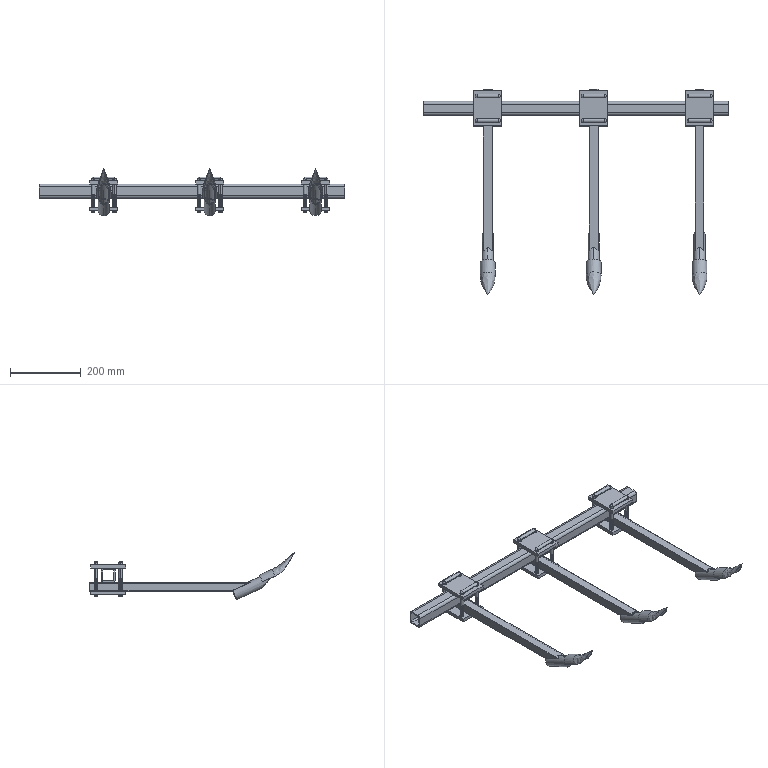Part | SolidWorks | 16 solids | 1299 faces | box 866 x 581.033 x 134.332 mm | volume 1380836 mm3 | cylinder 1112 | plane 127 | spline 48 | sphere 12 | commonest cylinder face diameters 10 x1032 11 x48 32 x15 28 x6 8 x4 16 x4